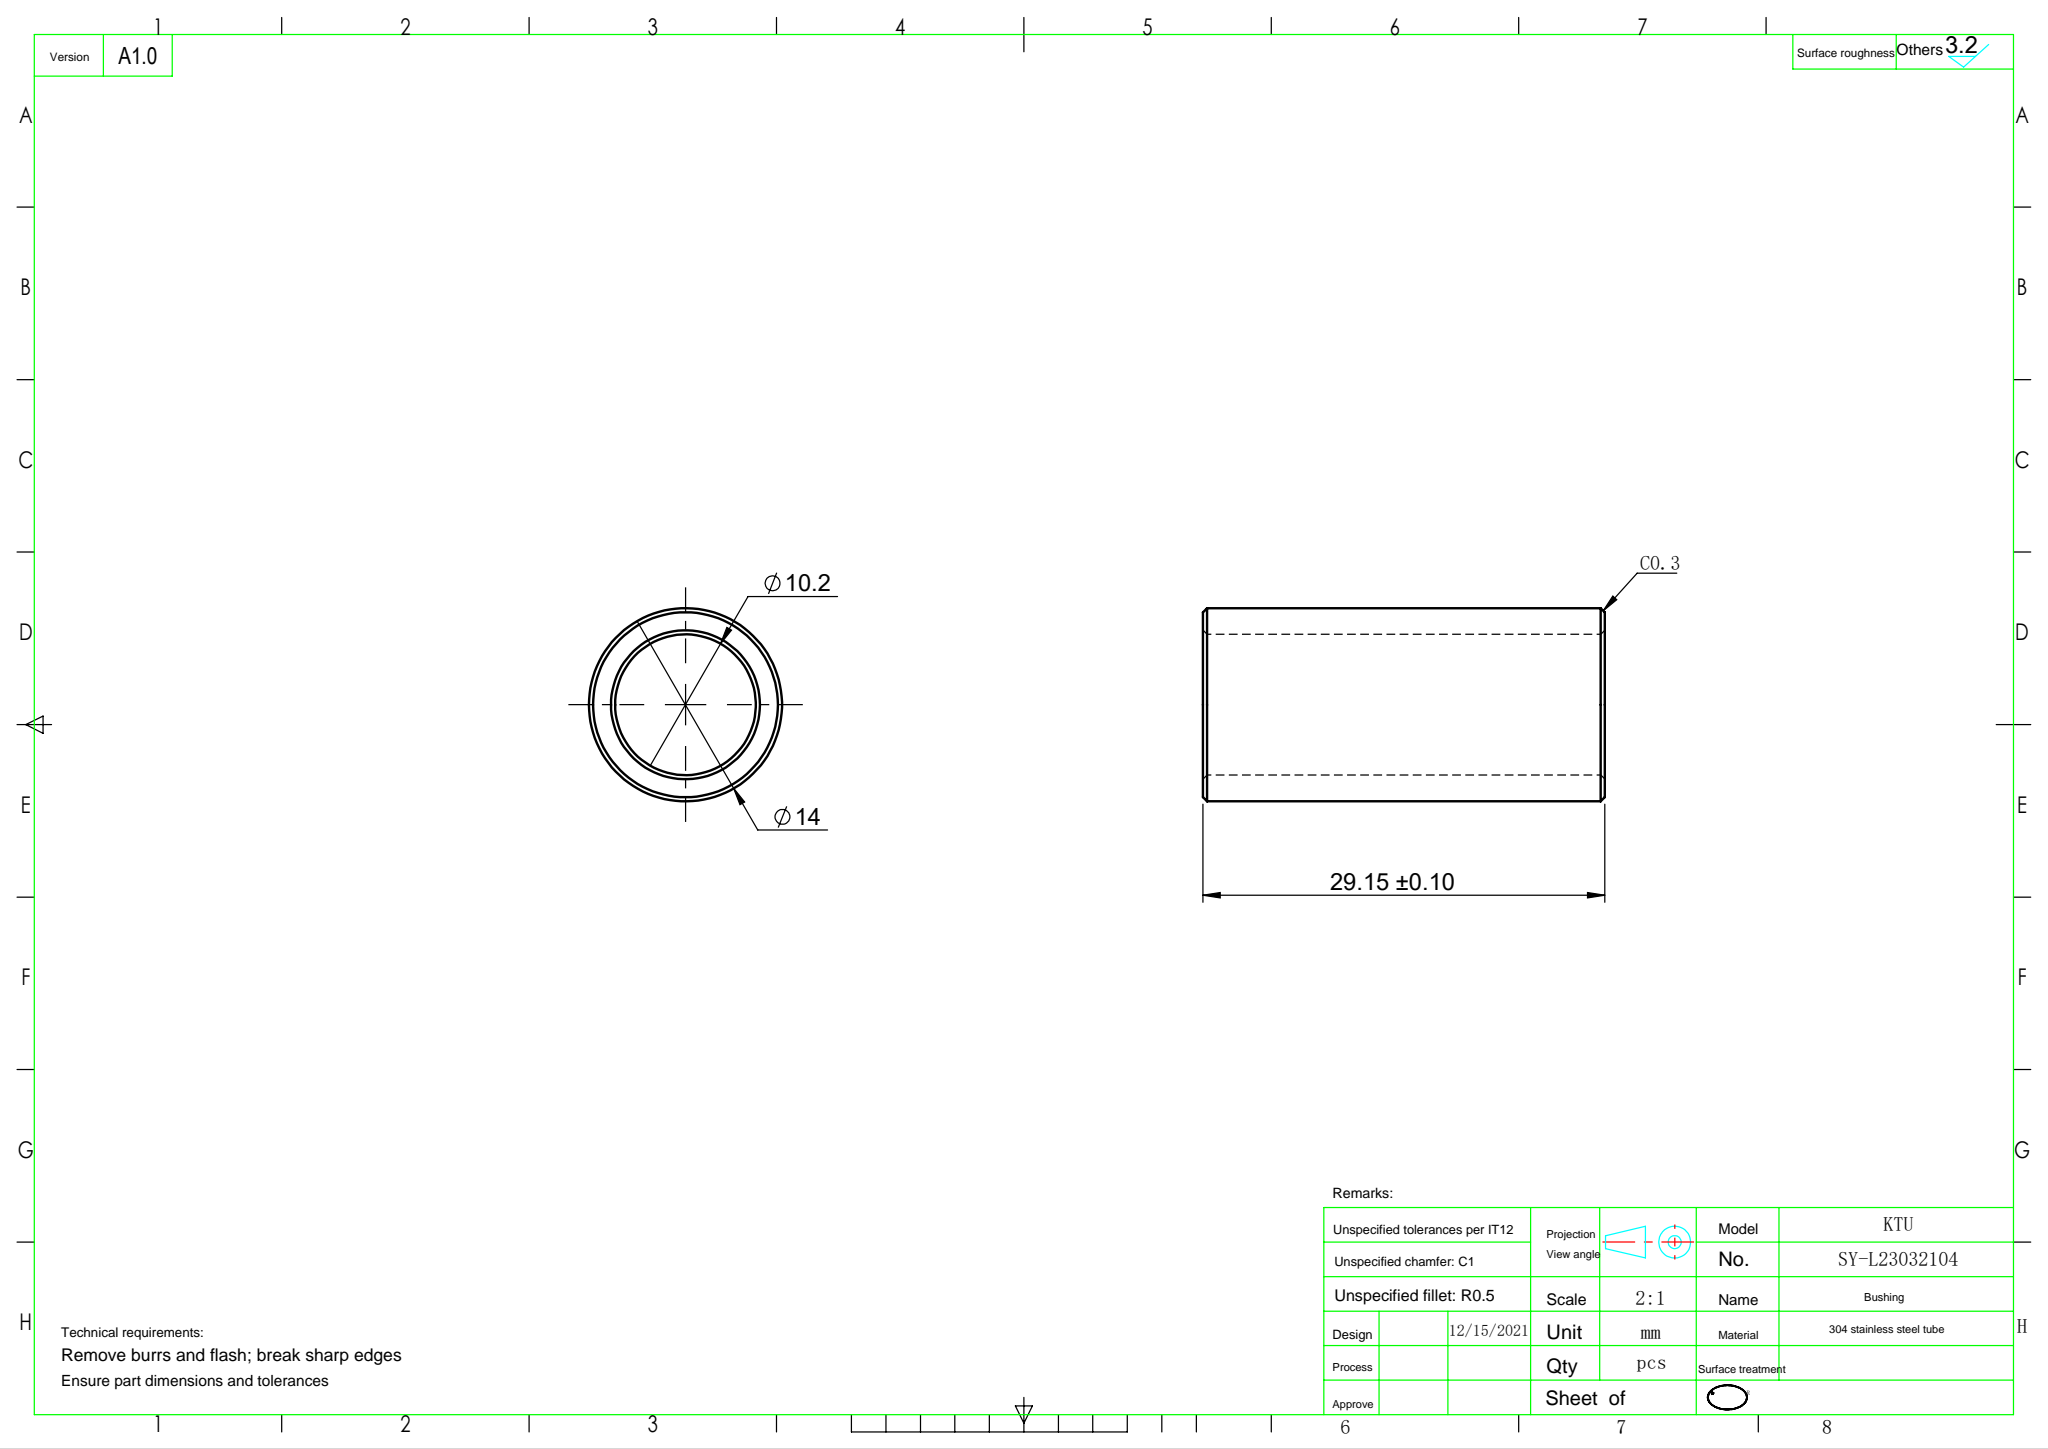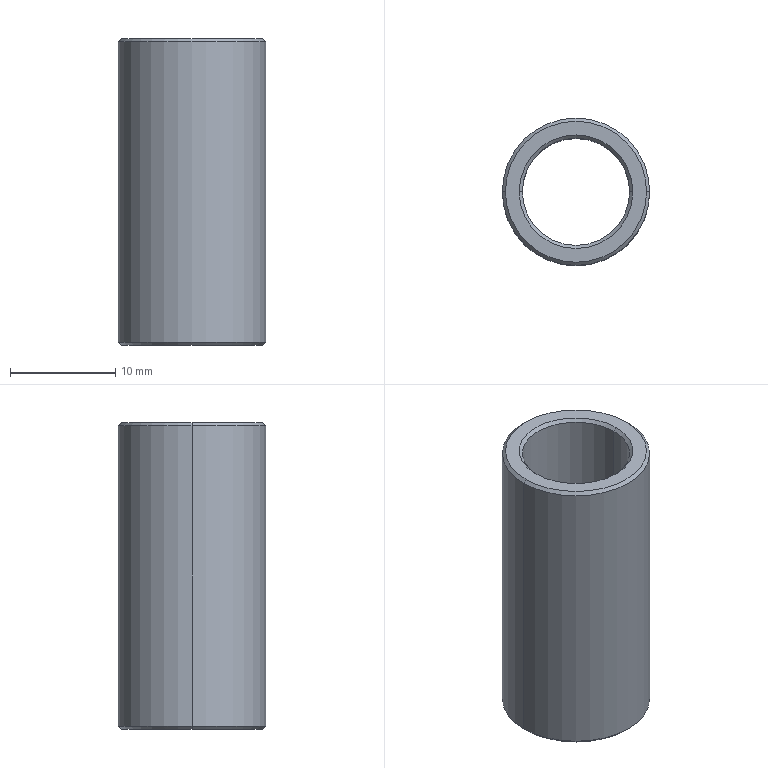Part | SolidWorks | features Chamfer 2, Extrusion 1 | 1 solid | 14 faces | box 14 x 14 x 29.15 mm | volume 2099 mm3 | cone 8 | cylinder 4 | plane 2 | commonest cylinder face diameters 10.2 x2 14 x2
STEP:
#1=CARTESIAN_POINT('',(6.7,0.,29.15));
#2=VERTEX_POINT('',#1);
#3=CARTESIAN_POINT('',(-6.7,0.,29.15));
#4=VERTEX_POINT('',#3);
#5=CARTESIAN_POINT('',(0.,0.,29.15));
#6=DIRECTION('',(0.,0.,1.));
#7=DIRECTION('',(1.,0.,0.));
#8=AXIS2_PLACEMENT_3D('',#5,#6,#7);
#9=CIRCLE('',#8,6.7);
#10=EDGE_CURVE('',#2,#4,#9,.T.);
#11=ORIENTED_EDGE('',*,*,#10,.F.);
#12=CARTESIAN_POINT('',(7.,0.,28.85));
#13=VERTEX_POINT('',#12);
#14=CARTESIAN_POINT('',(6.7,0.,29.15));
#15=DIRECTION('',(0.7071,0.,-0.7071));
#16=VECTOR('',#15,1000.);
#17=LINE('',#14,#16);
#18=EDGE_CURVE('',#2,#13,#17,.T.);
#19=ORIENTED_EDGE('',*,*,#18,.T.);
#20=CARTESIAN_POINT('',(-7.,0.,28.85));
#21=VERTEX_POINT('',#20);
#22=CARTESIAN_POINT('',(0.,0.,28.85));
#23=DIRECTION('',(0.,0.,-1.));
#24=DIRECTION('',(1.,0.,0.));
#25=AXIS2_PLACEMENT_3D('',#22,#23,#24);
#26=CIRCLE('',#25,7.);
#27=EDGE_CURVE('',#21,#13,#26,.T.);
#28=ORIENTED_EDGE('',*,*,#27,.F.);
#29=CARTESIAN_POINT('',(-6.7,0.,29.15));
#30=DIRECTION('',(-0.7071,0.,-0.7071));
#31=VECTOR('',#30,1000.);
#32=LINE('',#29,#31);
#33=EDGE_CURVE('',#4,#21,#32,.T.);
#34=ORIENTED_EDGE('',*,*,#33,.F.);
#35=EDGE_LOOP('',(#11,#19,#28,#34));
#36=FACE_OUTER_BOUND('',#35,.T.);
#37=CARTESIAN_POINT('',(0.,0.,29.15));
#38=DIRECTION('',(0.,0.,-1.));
#39=DIRECTION('',(-1.,0.,0.));
#40=AXIS2_PLACEMENT_3D('',#37,#38,#39);
#41=CONICAL_SURFACE('',#40,6.7,0.7854);
#42=ADVANCED_FACE('',(#36),#41,.T.);
#43=CARTESIAN_POINT('',(-5.1,0.,28.85));
#44=VERTEX_POINT('',#43);
#45=CARTESIAN_POINT('',(5.1,0.,28.85));
#46=VERTEX_POINT('',#45);
#47=CARTESIAN_POINT('',(0.,0.,28.85));
#48=DIRECTION('',(0.,0.,1.));
#49=DIRECTION('',(1.,0.,0.));
#50=AXIS2_PLACEMENT_3D('',#47,#48,#49);
#51=CIRCLE('',#50,5.1);
#52=EDGE_CURVE('',#44,#46,#51,.T.);
#53=ORIENTED_EDGE('',*,*,#52,.F.);
#54=CARTESIAN_POINT('',(-5.4,0.,29.15));
#55=VERTEX_POINT('',#54);
#56=CARTESIAN_POINT('',(-5.1,0.,28.85));
#57=DIRECTION('',(-0.7071,0.,0.7071));
#58=VECTOR('',#57,1000.);
#59=LINE('',#56,#58);
#60=EDGE_CURVE('',#44,#55,#59,.T.);
#61=ORIENTED_EDGE('',*,*,#60,.T.);
#62=CARTESIAN_POINT('',(5.4,0.,29.15));
#63=VERTEX_POINT('',#62);
#64=CARTESIAN_POINT('',(0.,0.,29.15));
#65=DIRECTION('',(0.,0.,-1.));
#66=DIRECTION('',(1.,0.,0.));
#67=AXIS2_PLACEMENT_3D('',#64,#65,#66);
#68=CIRCLE('',#67,5.4);
#69=EDGE_CURVE('',#63,#55,#68,.T.);
#70=ORIENTED_EDGE('',*,*,#69,.F.);
#71=CARTESIAN_POINT('',(5.1,0.,28.85));
#72=DIRECTION('',(0.7071,0.,0.7071));
#73=VECTOR('',#72,1000.);
#74=LINE('',#71,#73);
#75=EDGE_CURVE('',#46,#63,#74,.T.);
#76=ORIENTED_EDGE('',*,*,#75,.F.);
#77=EDGE_LOOP('',(#53,#61,#70,#76));
#78=FACE_OUTER_BOUND('',#77,.T.);
#79=CARTESIAN_POINT('',(0.,0.,28.85));
#80=DIRECTION('',(0.,0.,1.));
#81=DIRECTION('',(1.,0.,0.));
#82=AXIS2_PLACEMENT_3D('',#79,#80,#81);
#83=CONICAL_SURFACE('',#82,5.1,0.7854);
#84=ADVANCED_FACE('',(#78),#83,.F.);
#85=CARTESIAN_POINT('',(5.1,0.,0.3));
#86=VERTEX_POINT('',#85);
#87=CARTESIAN_POINT('',(-5.1,0.,0.3));
#88=VERTEX_POINT('',#87);
#89=CARTESIAN_POINT('',(0.,0.,0.3));
#90=DIRECTION('',(0.,0.,-1.));
#91=DIRECTION('',(1.,0.,0.));
#92=AXIS2_PLACEMENT_3D('',#89,#90,#91);
#93=CIRCLE('',#92,5.1);
#94=EDGE_CURVE('',#86,#88,#93,.T.);
#95=ORIENTED_EDGE('',*,*,#94,.F.);
#96=CARTESIAN_POINT('',(5.4,0.,0.));
#97=VERTEX_POINT('',#96);
#98=CARTESIAN_POINT('',(5.4,0.,0.));
#99=DIRECTION('',(0.7071,0.,-0.7071));
#100=VECTOR('',#99,1000.);
#101=LINE('',#98,#100);
#102=EDGE_CURVE('',#86,#97,#101,.T.);
#103=ORIENTED_EDGE('',*,*,#102,.T.);
#104=CARTESIAN_POINT('',(-5.4,0.,0.));
#105=VERTEX_POINT('',#104);
#106=CARTESIAN_POINT('',(0.,0.,0.));
#107=DIRECTION('',(0.,0.,1.));
#108=DIRECTION('',(1.,0.,0.));
#109=AXIS2_PLACEMENT_3D('',#106,#107,#108);
#110=CIRCLE('',#109,5.4);
#111=EDGE_CURVE('',#105,#97,#110,.T.);
#112=ORIENTED_EDGE('',*,*,#111,.F.);
#113=CARTESIAN_POINT('',(-5.4,0.,0.));
#114=DIRECTION('',(-0.7071,0.,-0.7071));
#115=VECTOR('',#114,1000.);
#116=LINE('',#113,#115);
#117=EDGE_CURVE('',#88,#105,#116,.T.);
#118=ORIENTED_EDGE('',*,*,#117,.F.);
#119=EDGE_LOOP('',(#95,#103,#112,#118));
#120=FACE_OUTER_BOUND('',#119,.T.);
#121=CARTESIAN_POINT('',(0.,0.,0.));
#122=DIRECTION('',(0.,0.,-1.));
#123=DIRECTION('',(-1.,0.,0.));
#124=AXIS2_PLACEMENT_3D('',#121,#122,#123);
#125=CONICAL_SURFACE('',#124,5.4,0.7854);
#126=ADVANCED_FACE('',(#120),#125,.F.);
#127=CARTESIAN_POINT('',(-6.7,0.,0.));
#128=VERTEX_POINT('',#127);
#129=CARTESIAN_POINT('',(6.7,0.,0.));
#130=VERTEX_POINT('',#129);
#131=CARTESIAN_POINT('',(0.,0.,0.));
#132=DIRECTION('',(0.,0.,-1.));
#133=DIRECTION('',(1.,0.,0.));
#134=AXIS2_PLACEMENT_3D('',#131,#132,#133);
#135=CIRCLE('',#134,6.7);
#136=EDGE_CURVE('',#128,#130,#135,.T.);
#137=ORIENTED_EDGE('',*,*,#136,.F.);
#138=CARTESIAN_POINT('',(-7.,0.,0.3));
#139=VERTEX_POINT('',#138);
#140=CARTESIAN_POINT('',(-7.,0.,0.3));
#141=DIRECTION('',(-0.7071,0.,0.7071));
#142=VECTOR('',#141,1000.);
#143=LINE('',#140,#142);
#144=EDGE_CURVE('',#128,#139,#143,.T.);
#145=ORIENTED_EDGE('',*,*,#144,.T.);
#146=CARTESIAN_POINT('',(7.,0.,0.3));
#147=VERTEX_POINT('',#146);
#148=CARTESIAN_POINT('',(0.,0.,0.3));
#149=DIRECTION('',(0.,0.,1.));
#150=DIRECTION('',(1.,0.,0.));
#151=AXIS2_PLACEMENT_3D('',#148,#149,#150);
#152=CIRCLE('',#151,7.);
#153=EDGE_CURVE('',#147,#139,#152,.T.);
#154=ORIENTED_EDGE('',*,*,#153,.F.);
#155=CARTESIAN_POINT('',(7.,0.,0.3));
#156=DIRECTION('',(0.7071,0.,0.7071));
#157=VECTOR('',#156,1000.);
#158=LINE('',#155,#157);
#159=EDGE_CURVE('',#130,#147,#158,.T.);
#160=ORIENTED_EDGE('',*,*,#159,.F.);
#161=EDGE_LOOP('',(#137,#145,#154,#160));
#162=FACE_OUTER_BOUND('',#161,.T.);
#163=CARTESIAN_POINT('',(0.,0.,0.3));
#164=DIRECTION('',(0.,0.,1.));
#165=DIRECTION('',(1.,0.,0.));
#166=AXIS2_PLACEMENT_3D('',#163,#164,#165);
#167=CONICAL_SURFACE('',#166,7.,0.7854);
#168=ADVANCED_FACE('',(#162),#167,.T.);
#169=ORIENTED_EDGE('',*,*,#52,.T.);
#170=CARTESIAN_POINT('',(5.1,0.,29.15));
#171=DIRECTION('',(0.,0.,-1.));
#172=VECTOR('',#171,1000.);
#173=LINE('',#170,#172);
#174=EDGE_CURVE('',#46,#86,#173,.T.);
#175=ORIENTED_EDGE('',*,*,#174,.T.);
#176=ORIENTED_EDGE('',*,*,#94,.T.);
#177=CARTESIAN_POINT('',(-5.1,0.,29.15));
#178=DIRECTION('',(0.,0.,-1.));
#179=VECTOR('',#178,1000.);
#180=LINE('',#177,#179);
#181=EDGE_CURVE('',#44,#88,#180,.T.);
#182=ORIENTED_EDGE('',*,*,#181,.F.);
#183=EDGE_LOOP('',(#169,#175,#176,#182));
#184=FACE_OUTER_BOUND('',#183,.T.);
#185=CARTESIAN_POINT('',(0.,0.,29.15));
#186=DIRECTION('',(0.,0.,-1.));
#187=DIRECTION('',(-1.,0.,0.));
#188=AXIS2_PLACEMENT_3D('',#185,#186,#187);
#189=CYLINDRICAL_SURFACE('',#188,5.1);
#190=ADVANCED_FACE('',(#184),#189,.F.);
#191=ORIENTED_EDGE('',*,*,#27,.T.);
#192=CARTESIAN_POINT('',(7.,0.,29.15));
#193=DIRECTION('',(0.,0.,-1.));
#194=VECTOR('',#193,1000.);
#195=LINE('',#192,#194);
#196=EDGE_CURVE('',#13,#147,#195,.T.);
#197=ORIENTED_EDGE('',*,*,#196,.T.);
#198=ORIENTED_EDGE('',*,*,#153,.T.);
#199=CARTESIAN_POINT('',(-7.,0.,29.15));
#200=DIRECTION('',(0.,0.,-1.));
#201=VECTOR('',#200,1000.);
#202=LINE('',#199,#201);
#203=EDGE_CURVE('',#21,#139,#202,.T.);
#204=ORIENTED_EDGE('',*,*,#203,.F.);
#205=EDGE_LOOP('',(#191,#197,#198,#204));
#206=FACE_OUTER_BOUND('',#205,.T.);
#207=CARTESIAN_POINT('',(0.,0.,29.15));
#208=DIRECTION('',(0.,0.,-1.));
#209=DIRECTION('',(-1.,0.,0.));
#210=AXIS2_PLACEMENT_3D('',#207,#208,#209);
#211=CYLINDRICAL_SURFACE('',#210,7.);
#212=ADVANCED_FACE('',(#206),#211,.T.);
#213=ORIENTED_EDGE('',*,*,#69,.T.);
#214=CARTESIAN_POINT('',(0.,0.,29.15));
#215=DIRECTION('',(0.,0.,-1.));
#216=DIRECTION('',(1.,0.,0.));
#217=AXIS2_PLACEMENT_3D('',#214,#215,#216);
#218=CIRCLE('',#217,5.4);
#219=EDGE_CURVE('',#55,#63,#218,.T.);
#220=ORIENTED_EDGE('',*,*,#219,.T.);
#221=EDGE_LOOP('',(#213,#220));
#222=FACE_BOUND('',#221,.T.);
#223=CARTESIAN_POINT('',(0.,0.,29.15));
#224=DIRECTION('',(0.,0.,1.));
#225=DIRECTION('',(1.,0.,0.));
#226=AXIS2_PLACEMENT_3D('',#223,#224,#225);
#227=CIRCLE('',#226,6.7);
#228=EDGE_CURVE('',#4,#2,#227,.T.);
#229=ORIENTED_EDGE('',*,*,#228,.T.);
#230=ORIENTED_EDGE('',*,*,#10,.T.);
#231=EDGE_LOOP('',(#229,#230));
#232=FACE_OUTER_BOUND('',#231,.T.);
#233=CARTESIAN_POINT('',(0.,0.,29.15));
#234=DIRECTION('',(0.,0.,1.));
#235=DIRECTION('',(1.,0.,0.));
#236=AXIS2_PLACEMENT_3D('',#233,#234,#235);
#237=PLANE('',#236);
#238=ADVANCED_FACE('',(#222,#232),#237,.T.);
#239=ORIENTED_EDGE('',*,*,#111,.T.);
#240=CARTESIAN_POINT('',(0.,0.,0.));
#241=DIRECTION('',(0.,0.,1.));
#242=DIRECTION('',(1.,0.,0.));
#243=AXIS2_PLACEMENT_3D('',#240,#241,#242);
#244=CIRCLE('',#243,5.4);
#245=EDGE_CURVE('',#97,#105,#244,.T.);
#246=ORIENTED_EDGE('',*,*,#245,.T.);
#247=EDGE_LOOP('',(#239,#246));
#248=FACE_BOUND('',#247,.T.);
#249=CARTESIAN_POINT('',(0.,0.,0.));
#250=DIRECTION('',(0.,0.,-1.));
#251=DIRECTION('',(1.,0.,0.));
#252=AXIS2_PLACEMENT_3D('',#249,#250,#251);
#253=CIRCLE('',#252,6.7);
#254=EDGE_CURVE('',#130,#128,#253,.T.);
#255=ORIENTED_EDGE('',*,*,#254,.T.);
#256=ORIENTED_EDGE('',*,*,#136,.T.);
#257=EDGE_LOOP('',(#255,#256));
#258=FACE_OUTER_BOUND('',#257,.T.);
#259=CARTESIAN_POINT('',(0.,0.,0.));
#260=DIRECTION('',(0.,0.,1.));
#261=DIRECTION('',(1.,0.,0.));
#262=AXIS2_PLACEMENT_3D('',#259,#260,#261);
#263=PLANE('',#262);
#264=ADVANCED_FACE('',(#248,#258),#263,.F.);
#265=ORIENTED_EDGE('',*,*,#196,.F.);
#266=CARTESIAN_POINT('',(0.,0.,28.85));
#267=DIRECTION('',(0.,0.,-1.));
#268=DIRECTION('',(1.,0.,0.));
#269=AXIS2_PLACEMENT_3D('',#266,#267,#268);
#270=CIRCLE('',#269,7.);
#271=EDGE_CURVE('',#13,#21,#270,.T.);
#272=ORIENTED_EDGE('',*,*,#271,.T.);
#273=ORIENTED_EDGE('',*,*,#203,.T.);
#274=CARTESIAN_POINT('',(0.,0.,0.3));
#275=DIRECTION('',(0.,0.,1.));
#276=DIRECTION('',(1.,0.,0.));
#277=AXIS2_PLACEMENT_3D('',#274,#275,#276);
#278=CIRCLE('',#277,7.);
#279=EDGE_CURVE('',#139,#147,#278,.T.);
#280=ORIENTED_EDGE('',*,*,#279,.T.);
#281=EDGE_LOOP('',(#265,#272,#273,#280));
#282=FACE_OUTER_BOUND('',#281,.T.);
#283=CARTESIAN_POINT('',(0.,0.,29.15));
#284=DIRECTION('',(0.,0.,-1.));
#285=DIRECTION('',(-1.,0.,0.));
#286=AXIS2_PLACEMENT_3D('',#283,#284,#285);
#287=CYLINDRICAL_SURFACE('',#286,7.);
#288=ADVANCED_FACE('',(#282),#287,.T.);
#289=ORIENTED_EDGE('',*,*,#174,.F.);
#290=CARTESIAN_POINT('',(0.,0.,28.85));
#291=DIRECTION('',(0.,0.,1.));
#292=DIRECTION('',(1.,0.,0.));
#293=AXIS2_PLACEMENT_3D('',#290,#291,#292);
#294=CIRCLE('',#293,5.1);
#295=EDGE_CURVE('',#46,#44,#294,.T.);
#296=ORIENTED_EDGE('',*,*,#295,.T.);
#297=ORIENTED_EDGE('',*,*,#181,.T.);
#298=CARTESIAN_POINT('',(0.,0.,0.3));
#299=DIRECTION('',(0.,0.,-1.));
#300=DIRECTION('',(1.,0.,0.));
#301=AXIS2_PLACEMENT_3D('',#298,#299,#300);
#302=CIRCLE('',#301,5.1);
#303=EDGE_CURVE('',#88,#86,#302,.T.);
#304=ORIENTED_EDGE('',*,*,#303,.T.);
#305=EDGE_LOOP('',(#289,#296,#297,#304));
#306=FACE_OUTER_BOUND('',#305,.T.);
#307=CARTESIAN_POINT('',(0.,0.,29.15));
#308=DIRECTION('',(0.,0.,-1.));
#309=DIRECTION('',(-1.,0.,0.));
#310=AXIS2_PLACEMENT_3D('',#307,#308,#309);
#311=CYLINDRICAL_SURFACE('',#310,5.1);
#312=ADVANCED_FACE('',(#306),#311,.F.);
#313=ORIENTED_EDGE('',*,*,#144,.F.);
#314=ORIENTED_EDGE('',*,*,#254,.F.);
#315=ORIENTED_EDGE('',*,*,#159,.T.);
#316=ORIENTED_EDGE('',*,*,#279,.F.);
#317=EDGE_LOOP('',(#313,#314,#315,#316));
#318=FACE_OUTER_BOUND('',#317,.T.);
#319=CARTESIAN_POINT('',(0.,0.,0.3));
#320=DIRECTION('',(0.,0.,1.));
#321=DIRECTION('',(1.,0.,0.));
#322=AXIS2_PLACEMENT_3D('',#319,#320,#321);
#323=CONICAL_SURFACE('',#322,7.,0.7854);
#324=ADVANCED_FACE('',(#318),#323,.T.);
#325=ORIENTED_EDGE('',*,*,#102,.F.);
#326=ORIENTED_EDGE('',*,*,#303,.F.);
#327=ORIENTED_EDGE('',*,*,#117,.T.);
#328=ORIENTED_EDGE('',*,*,#245,.F.);
#329=EDGE_LOOP('',(#325,#326,#327,#328));
#330=FACE_OUTER_BOUND('',#329,.T.);
#331=CARTESIAN_POINT('',(0.,0.,0.));
#332=DIRECTION('',(0.,0.,-1.));
#333=DIRECTION('',(-1.,0.,0.));
#334=AXIS2_PLACEMENT_3D('',#331,#332,#333);
#335=CONICAL_SURFACE('',#334,5.4,0.7854);
#336=ADVANCED_FACE('',(#330),#335,.F.);
#337=ORIENTED_EDGE('',*,*,#60,.F.);
#338=ORIENTED_EDGE('',*,*,#295,.F.);
#339=ORIENTED_EDGE('',*,*,#75,.T.);
#340=ORIENTED_EDGE('',*,*,#219,.F.);
#341=EDGE_LOOP('',(#337,#338,#339,#340));
#342=FACE_OUTER_BOUND('',#341,.T.);
#343=CARTESIAN_POINT('',(0.,0.,28.85));
#344=DIRECTION('',(0.,0.,1.));
#345=DIRECTION('',(1.,0.,0.));
#346=AXIS2_PLACEMENT_3D('',#343,#344,#345);
#347=CONICAL_SURFACE('',#346,5.1,0.7854);
#348=ADVANCED_FACE('',(#342),#347,.F.);
#349=ORIENTED_EDGE('',*,*,#18,.F.);
#350=ORIENTED_EDGE('',*,*,#228,.F.);
#351=ORIENTED_EDGE('',*,*,#33,.T.);
#352=ORIENTED_EDGE('',*,*,#271,.F.);
#353=EDGE_LOOP('',(#349,#350,#351,#352));
#354=FACE_OUTER_BOUND('',#353,.T.);
#355=CARTESIAN_POINT('',(0.,0.,29.15));
#356=DIRECTION('',(0.,0.,-1.));
#357=DIRECTION('',(-1.,0.,0.));
#358=AXIS2_PLACEMENT_3D('',#355,#356,#357);
#359=CONICAL_SURFACE('',#358,6.7,0.7854);
#360=ADVANCED_FACE('',(#354),#359,.T.);
#361=CLOSED_SHELL('',(#42,#84,#126,#168,#190,#212,#238,#264,#288,#312,#324,#336,#348,#360));
#362=MANIFOLD_SOLID_BREP('',#361);
#363=CARTESIAN_POINT('',(0.,0.,0.));
#364=DIRECTION('',(0.,0.,1.));
#365=DIRECTION('',(1.,0.,0.));
#366=AXIS2_PLACEMENT_3D('',#363,#364,#365);
#367=(LENGTH_UNIT()NAMED_UNIT(*)SI_UNIT(.MILLI.,.METRE.));
#368=UNCERTAINTY_MEASURE_WITH_UNIT(LENGTH_MEASURE(0.00001),#367,'','');
#369=(NAMED_UNIT(*)PLANE_ANGLE_UNIT()SI_UNIT($,.RADIAN.));
#370=(NAMED_UNIT(*)SI_UNIT($,.STERADIAN.)SOLID_ANGLE_UNIT());
#371=(GEOMETRIC_REPRESENTATION_CONTEXT(3)GLOBAL_UNCERTAINTY_ASSIGNED_CONTEXT((#368))GLOBAL_UNIT_ASSIGNED_CONTEXT((#367,#369,#370))REPRESENTATION_CONTEXT('',''));
#372=ADVANCED_BREP_SHAPE_REPRESENTATION('',(#362,#366),#371);